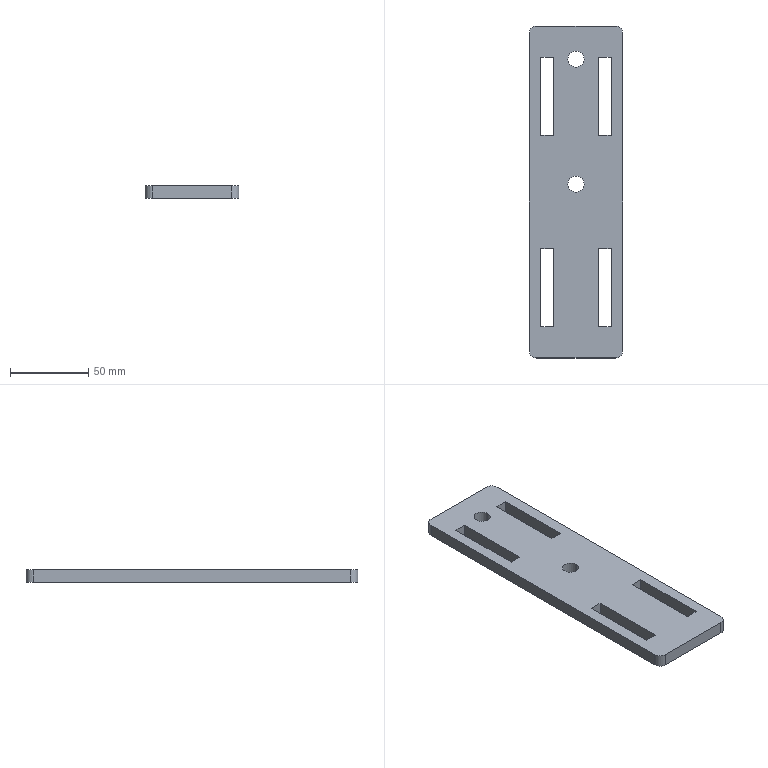Part | SolidWorks | features FlatPattern 1, SMBaseFlange 1, SheetMetal 1 | 1 solid | 30 faces | box 60 x 212.5 x 8 mm | volume 87695 mm3 | plane 22 | cylinder 8 | commonest cylinder face diameters 10 x4 10.3 x4
STEP:
#1=CARTESIAN_POINT('',(326.222,40.247,-8.));
#2=VERTEX_POINT('',#1);
#3=CARTESIAN_POINT('',(336.522,40.247,-8.));
#4=VERTEX_POINT('',#3);
#5=CARTESIAN_POINT('',(331.372,40.247,-8.));
#6=DIRECTION('',(0.,0.,1.));
#7=DIRECTION('',(1.,0.,0.));
#8=AXIS2_PLACEMENT_3D('',#5,#6,#7);
#9=CIRCLE('',#8,5.15);
#10=EDGE_CURVE('',#2,#4,#9,.T.);
#11=ORIENTED_EDGE('',*,*,#10,.F.);
#12=CARTESIAN_POINT('',(326.222,40.247,0.));
#13=VERTEX_POINT('',#12);
#14=CARTESIAN_POINT('',(326.222,40.247,-8.));
#15=DIRECTION('',(0.,0.,1.));
#16=VECTOR('',#15,1000.);
#17=LINE('',#14,#16);
#18=EDGE_CURVE('',#2,#13,#17,.T.);
#19=ORIENTED_EDGE('',*,*,#18,.T.);
#20=CARTESIAN_POINT('',(336.522,40.247,0.));
#21=VERTEX_POINT('',#20);
#22=CARTESIAN_POINT('',(331.372,40.247,0.));
#23=DIRECTION('',(0.,0.,1.));
#24=DIRECTION('',(1.,0.,0.));
#25=AXIS2_PLACEMENT_3D('',#22,#23,#24);
#26=CIRCLE('',#25,5.15);
#27=EDGE_CURVE('',#13,#21,#26,.T.);
#28=ORIENTED_EDGE('',*,*,#27,.T.);
#29=CARTESIAN_POINT('',(336.522,40.247,-8.));
#30=DIRECTION('',(0.,0.,1.));
#31=VECTOR('',#30,1000.);
#32=LINE('',#29,#31);
#33=EDGE_CURVE('',#4,#21,#32,.T.);
#34=ORIENTED_EDGE('',*,*,#33,.F.);
#35=EDGE_LOOP('',(#11,#19,#28,#34));
#36=FACE_OUTER_BOUND('',#35,.T.);
#37=CARTESIAN_POINT('',(331.372,40.247,-8.));
#38=DIRECTION('',(0.,0.,1.));
#39=DIRECTION('',(1.,0.,0.));
#40=AXIS2_PLACEMENT_3D('',#37,#38,#39);
#41=CYLINDRICAL_SURFACE('',#40,5.15);
#42=ADVANCED_FACE('',(#36),#41,.F.);
#43=CARTESIAN_POINT('',(326.222,-39.753,-8.));
#44=VERTEX_POINT('',#43);
#45=CARTESIAN_POINT('',(336.522,-39.753,-8.));
#46=VERTEX_POINT('',#45);
#47=CARTESIAN_POINT('',(331.372,-39.753,-8.));
#48=DIRECTION('',(0.,0.,1.));
#49=DIRECTION('',(1.,0.,0.));
#50=AXIS2_PLACEMENT_3D('',#47,#48,#49);
#51=CIRCLE('',#50,5.15);
#52=EDGE_CURVE('',#44,#46,#51,.T.);
#53=ORIENTED_EDGE('',*,*,#52,.F.);
#54=CARTESIAN_POINT('',(326.222,-39.753,0.));
#55=VERTEX_POINT('',#54);
#56=CARTESIAN_POINT('',(326.222,-39.753,-8.));
#57=DIRECTION('',(0.,0.,1.));
#58=VECTOR('',#57,1000.);
#59=LINE('',#56,#58);
#60=EDGE_CURVE('',#44,#55,#59,.T.);
#61=ORIENTED_EDGE('',*,*,#60,.T.);
#62=CARTESIAN_POINT('',(336.522,-39.753,0.));
#63=VERTEX_POINT('',#62);
#64=CARTESIAN_POINT('',(331.372,-39.753,0.));
#65=DIRECTION('',(0.,0.,1.));
#66=DIRECTION('',(1.,0.,0.));
#67=AXIS2_PLACEMENT_3D('',#64,#65,#66);
#68=CIRCLE('',#67,5.15);
#69=EDGE_CURVE('',#55,#63,#68,.T.);
#70=ORIENTED_EDGE('',*,*,#69,.T.);
#71=CARTESIAN_POINT('',(336.522,-39.753,-8.));
#72=DIRECTION('',(0.,0.,1.));
#73=VECTOR('',#72,1000.);
#74=LINE('',#71,#73);
#75=EDGE_CURVE('',#46,#63,#74,.T.);
#76=ORIENTED_EDGE('',*,*,#75,.F.);
#77=EDGE_LOOP('',(#53,#61,#70,#76));
#78=FACE_OUTER_BOUND('',#77,.T.);
#79=CARTESIAN_POINT('',(331.372,-39.753,-8.));
#80=DIRECTION('',(0.,0.,1.));
#81=DIRECTION('',(1.,0.,0.));
#82=AXIS2_PLACEMENT_3D('',#79,#80,#81);
#83=CYLINDRICAL_SURFACE('',#82,5.15);
#84=ADVANCED_FACE('',(#78),#83,.F.);
#85=CARTESIAN_POINT('',(356.372,-151.003,0.));
#86=VERTEX_POINT('',#85);
#87=CARTESIAN_POINT('',(361.372,-146.003,0.));
#88=VERTEX_POINT('',#87);
#89=CARTESIAN_POINT('',(356.372,-146.003,0.));
#90=DIRECTION('',(0.,0.,1.));
#91=DIRECTION('',(1.,0.,0.));
#92=AXIS2_PLACEMENT_3D('',#89,#90,#91);
#93=CIRCLE('',#92,5.);
#94=EDGE_CURVE('',#86,#88,#93,.T.);
#95=ORIENTED_EDGE('',*,*,#94,.F.);
#96=CARTESIAN_POINT('',(356.372,-151.003,-8.));
#97=VERTEX_POINT('',#96);
#98=CARTESIAN_POINT('',(356.372,-151.003,-8.));
#99=DIRECTION('',(0.,0.,1.));
#100=VECTOR('',#99,1000.);
#101=LINE('',#98,#100);
#102=EDGE_CURVE('',#97,#86,#101,.T.);
#103=ORIENTED_EDGE('',*,*,#102,.F.);
#104=CARTESIAN_POINT('',(361.372,-146.003,-8.));
#105=VERTEX_POINT('',#104);
#106=CARTESIAN_POINT('',(356.372,-146.003,-8.));
#107=DIRECTION('',(0.,0.,1.));
#108=DIRECTION('',(1.,0.,0.));
#109=AXIS2_PLACEMENT_3D('',#106,#107,#108);
#110=CIRCLE('',#109,5.);
#111=EDGE_CURVE('',#97,#105,#110,.T.);
#112=ORIENTED_EDGE('',*,*,#111,.T.);
#113=CARTESIAN_POINT('',(361.372,-146.003,-8.));
#114=DIRECTION('',(0.,0.,1.));
#115=VECTOR('',#114,1000.);
#116=LINE('',#113,#115);
#117=EDGE_CURVE('',#105,#88,#116,.T.);
#118=ORIENTED_EDGE('',*,*,#117,.T.);
#119=EDGE_LOOP('',(#95,#103,#112,#118));
#120=FACE_OUTER_BOUND('',#119,.T.);
#121=CARTESIAN_POINT('',(356.372,-146.003,-8.));
#122=DIRECTION('',(0.,0.,1.));
#123=DIRECTION('',(1.,0.,0.));
#124=AXIS2_PLACEMENT_3D('',#121,#122,#123);
#125=CYLINDRICAL_SURFACE('',#124,5.);
#126=ADVANCED_FACE('',(#120),#125,.T.);
#127=CARTESIAN_POINT('',(306.372,-151.003,0.));
#128=VERTEX_POINT('',#127);
#129=CARTESIAN_POINT('',(306.372,-151.003,0.));
#130=DIRECTION('',(1.,0.,0.));
#131=VECTOR('',#130,1000.);
#132=LINE('',#129,#131);
#133=EDGE_CURVE('',#128,#86,#132,.T.);
#134=ORIENTED_EDGE('',*,*,#133,.F.);
#135=CARTESIAN_POINT('',(306.372,-151.003,-8.));
#136=VERTEX_POINT('',#135);
#137=CARTESIAN_POINT('',(306.372,-151.003,-8.));
#138=DIRECTION('',(0.,0.,1.));
#139=VECTOR('',#138,1000.);
#140=LINE('',#137,#139);
#141=EDGE_CURVE('',#136,#128,#140,.T.);
#142=ORIENTED_EDGE('',*,*,#141,.F.);
#143=CARTESIAN_POINT('',(306.372,-151.003,-8.));
#144=DIRECTION('',(1.,0.,0.));
#145=VECTOR('',#144,1000.);
#146=LINE('',#143,#145);
#147=EDGE_CURVE('',#136,#97,#146,.T.);
#148=ORIENTED_EDGE('',*,*,#147,.T.);
#149=ORIENTED_EDGE('',*,*,#102,.T.);
#150=EDGE_LOOP('',(#134,#142,#148,#149));
#151=FACE_OUTER_BOUND('',#150,.T.);
#152=CARTESIAN_POINT('',(306.372,-151.003,-8.));
#153=DIRECTION('',(0.,-1.,0.));
#154=DIRECTION('',(1.,0.,0.));
#155=AXIS2_PLACEMENT_3D('',#152,#153,#154);
#156=PLANE('',#155);
#157=ADVANCED_FACE('',(#151),#156,.T.);
#158=CARTESIAN_POINT('',(301.372,-146.003,0.));
#159=VERTEX_POINT('',#158);
#160=CARTESIAN_POINT('',(306.372,-146.003,0.));
#161=DIRECTION('',(0.,0.,1.));
#162=DIRECTION('',(-1.,0.,0.));
#163=AXIS2_PLACEMENT_3D('',#160,#161,#162);
#164=CIRCLE('',#163,5.);
#165=EDGE_CURVE('',#159,#128,#164,.T.);
#166=ORIENTED_EDGE('',*,*,#165,.F.);
#167=CARTESIAN_POINT('',(301.372,-146.003,-8.));
#168=VERTEX_POINT('',#167);
#169=CARTESIAN_POINT('',(301.372,-146.003,-8.));
#170=DIRECTION('',(0.,0.,1.));
#171=VECTOR('',#170,1000.);
#172=LINE('',#169,#171);
#173=EDGE_CURVE('',#168,#159,#172,.T.);
#174=ORIENTED_EDGE('',*,*,#173,.F.);
#175=CARTESIAN_POINT('',(306.372,-146.003,-8.));
#176=DIRECTION('',(0.,0.,1.));
#177=DIRECTION('',(-1.,0.,0.));
#178=AXIS2_PLACEMENT_3D('',#175,#176,#177);
#179=CIRCLE('',#178,5.);
#180=EDGE_CURVE('',#168,#136,#179,.T.);
#181=ORIENTED_EDGE('',*,*,#180,.T.);
#182=ORIENTED_EDGE('',*,*,#141,.T.);
#183=EDGE_LOOP('',(#166,#174,#181,#182));
#184=FACE_OUTER_BOUND('',#183,.T.);
#185=CARTESIAN_POINT('',(306.372,-146.003,-8.));
#186=DIRECTION('',(0.,0.,1.));
#187=DIRECTION('',(1.,0.,0.));
#188=AXIS2_PLACEMENT_3D('',#185,#186,#187);
#189=CYLINDRICAL_SURFACE('',#188,5.);
#190=ADVANCED_FACE('',(#184),#189,.T.);
#191=CARTESIAN_POINT('',(301.372,56.497,0.));
#192=VERTEX_POINT('',#191);
#193=CARTESIAN_POINT('',(301.372,-146.003,0.));
#194=DIRECTION('',(0.,-1.,0.));
#195=VECTOR('',#194,1000.);
#196=LINE('',#193,#195);
#197=EDGE_CURVE('',#192,#159,#196,.T.);
#198=ORIENTED_EDGE('',*,*,#197,.F.);
#199=CARTESIAN_POINT('',(301.372,56.497,-8.));
#200=VERTEX_POINT('',#199);
#201=CARTESIAN_POINT('',(301.372,56.497,-8.));
#202=DIRECTION('',(0.,0.,1.));
#203=VECTOR('',#202,1000.);
#204=LINE('',#201,#203);
#205=EDGE_CURVE('',#200,#192,#204,.T.);
#206=ORIENTED_EDGE('',*,*,#205,.F.);
#207=CARTESIAN_POINT('',(301.372,-146.003,-8.));
#208=DIRECTION('',(0.,-1.,0.));
#209=VECTOR('',#208,1000.);
#210=LINE('',#207,#209);
#211=EDGE_CURVE('',#200,#168,#210,.T.);
#212=ORIENTED_EDGE('',*,*,#211,.T.);
#213=ORIENTED_EDGE('',*,*,#173,.T.);
#214=EDGE_LOOP('',(#198,#206,#212,#213));
#215=FACE_OUTER_BOUND('',#214,.T.);
#216=CARTESIAN_POINT('',(301.372,-146.003,-8.));
#217=DIRECTION('',(-1.,0.,0.));
#218=DIRECTION('',(0.,0.,1.));
#219=AXIS2_PLACEMENT_3D('',#216,#217,#218);
#220=PLANE('',#219);
#221=ADVANCED_FACE('',(#215),#220,.T.);
#222=CARTESIAN_POINT('',(306.372,61.497,0.));
#223=VERTEX_POINT('',#222);
#224=CARTESIAN_POINT('',(306.372,56.497,0.));
#225=DIRECTION('',(0.,0.,1.));
#226=DIRECTION('',(-1.,0.,0.));
#227=AXIS2_PLACEMENT_3D('',#224,#225,#226);
#228=CIRCLE('',#227,5.);
#229=EDGE_CURVE('',#223,#192,#228,.T.);
#230=ORIENTED_EDGE('',*,*,#229,.F.);
#231=CARTESIAN_POINT('',(306.372,61.497,-8.));
#232=VERTEX_POINT('',#231);
#233=CARTESIAN_POINT('',(306.372,61.497,-8.));
#234=DIRECTION('',(0.,0.,1.));
#235=VECTOR('',#234,1000.);
#236=LINE('',#233,#235);
#237=EDGE_CURVE('',#232,#223,#236,.T.);
#238=ORIENTED_EDGE('',*,*,#237,.F.);
#239=CARTESIAN_POINT('',(306.372,56.497,-8.));
#240=DIRECTION('',(0.,0.,1.));
#241=DIRECTION('',(-1.,0.,0.));
#242=AXIS2_PLACEMENT_3D('',#239,#240,#241);
#243=CIRCLE('',#242,5.);
#244=EDGE_CURVE('',#232,#200,#243,.T.);
#245=ORIENTED_EDGE('',*,*,#244,.T.);
#246=ORIENTED_EDGE('',*,*,#205,.T.);
#247=EDGE_LOOP('',(#230,#238,#245,#246));
#248=FACE_OUTER_BOUND('',#247,.T.);
#249=CARTESIAN_POINT('',(306.372,56.497,-8.));
#250=DIRECTION('',(0.,0.,1.));
#251=DIRECTION('',(1.,0.,0.));
#252=AXIS2_PLACEMENT_3D('',#249,#250,#251);
#253=CYLINDRICAL_SURFACE('',#252,5.);
#254=ADVANCED_FACE('',(#248),#253,.T.);
#255=CARTESIAN_POINT('',(356.372,61.497,0.));
#256=VERTEX_POINT('',#255);
#257=CARTESIAN_POINT('',(306.372,61.497,0.));
#258=DIRECTION('',(-1.,0.,0.));
#259=VECTOR('',#258,1000.);
#260=LINE('',#257,#259);
#261=EDGE_CURVE('',#256,#223,#260,.T.);
#262=ORIENTED_EDGE('',*,*,#261,.F.);
#263=CARTESIAN_POINT('',(356.372,61.497,-8.));
#264=VERTEX_POINT('',#263);
#265=CARTESIAN_POINT('',(356.372,61.497,-8.));
#266=DIRECTION('',(0.,0.,1.));
#267=VECTOR('',#266,1000.);
#268=LINE('',#265,#267);
#269=EDGE_CURVE('',#264,#256,#268,.T.);
#270=ORIENTED_EDGE('',*,*,#269,.F.);
#271=CARTESIAN_POINT('',(306.372,61.497,-8.));
#272=DIRECTION('',(-1.,0.,0.));
#273=VECTOR('',#272,1000.);
#274=LINE('',#271,#273);
#275=EDGE_CURVE('',#264,#232,#274,.T.);
#276=ORIENTED_EDGE('',*,*,#275,.T.);
#277=ORIENTED_EDGE('',*,*,#237,.T.);
#278=EDGE_LOOP('',(#262,#270,#276,#277));
#279=FACE_OUTER_BOUND('',#278,.T.);
#280=CARTESIAN_POINT('',(306.372,61.497,-8.));
#281=DIRECTION('',(0.,1.,0.));
#282=DIRECTION('',(0.,0.,1.));
#283=AXIS2_PLACEMENT_3D('',#280,#281,#282);
#284=PLANE('',#283);
#285=ADVANCED_FACE('',(#279),#284,.T.);
#286=CARTESIAN_POINT('',(361.372,56.497,0.));
#287=VERTEX_POINT('',#286);
#288=CARTESIAN_POINT('',(356.372,56.497,0.));
#289=DIRECTION('',(0.,0.,1.));
#290=DIRECTION('',(-1.,0.,0.));
#291=AXIS2_PLACEMENT_3D('',#288,#289,#290);
#292=CIRCLE('',#291,5.);
#293=EDGE_CURVE('',#287,#256,#292,.T.);
#294=ORIENTED_EDGE('',*,*,#293,.F.);
#295=CARTESIAN_POINT('',(361.372,56.497,-8.));
#296=VERTEX_POINT('',#295);
#297=CARTESIAN_POINT('',(361.372,56.497,-8.));
#298=DIRECTION('',(0.,0.,1.));
#299=VECTOR('',#298,1000.);
#300=LINE('',#297,#299);
#301=EDGE_CURVE('',#296,#287,#300,.T.);
#302=ORIENTED_EDGE('',*,*,#301,.F.);
#303=CARTESIAN_POINT('',(356.372,56.497,-8.));
#304=DIRECTION('',(0.,0.,1.));
#305=DIRECTION('',(-1.,0.,0.));
#306=AXIS2_PLACEMENT_3D('',#303,#304,#305);
#307=CIRCLE('',#306,5.);
#308=EDGE_CURVE('',#296,#264,#307,.T.);
#309=ORIENTED_EDGE('',*,*,#308,.T.);
#310=ORIENTED_EDGE('',*,*,#269,.T.);
#311=EDGE_LOOP('',(#294,#302,#309,#310));
#312=FACE_OUTER_BOUND('',#311,.T.);
#313=CARTESIAN_POINT('',(356.372,56.497,-8.));
#314=DIRECTION('',(0.,0.,1.));
#315=DIRECTION('',(1.,0.,0.));
#316=AXIS2_PLACEMENT_3D('',#313,#314,#315);
#317=CYLINDRICAL_SURFACE('',#316,5.);
#318=ADVANCED_FACE('',(#312),#317,.T.);
#319=CARTESIAN_POINT('',(361.372,-146.003,0.));
#320=DIRECTION('',(0.,1.,0.));
#321=VECTOR('',#320,1000.);
#322=LINE('',#319,#321);
#323=EDGE_CURVE('',#88,#287,#322,.T.);
#324=ORIENTED_EDGE('',*,*,#323,.F.);
#325=ORIENTED_EDGE('',*,*,#117,.F.);
#326=CARTESIAN_POINT('',(361.372,-146.003,-8.));
#327=DIRECTION('',(0.,1.,0.));
#328=VECTOR('',#327,1000.);
#329=LINE('',#326,#328);
#330=EDGE_CURVE('',#105,#296,#329,.T.);
#331=ORIENTED_EDGE('',*,*,#330,.T.);
#332=ORIENTED_EDGE('',*,*,#301,.T.);
#333=EDGE_LOOP('',(#324,#325,#331,#332));
#334=FACE_OUTER_BOUND('',#333,.T.);
#335=CARTESIAN_POINT('',(361.372,-146.003,-8.));
#336=DIRECTION('',(1.,0.,0.));
#337=DIRECTION('',(0.,0.,-1.));
#338=AXIS2_PLACEMENT_3D('',#335,#336,#337);
#339=PLANE('',#338);
#340=ADVANCED_FACE('',(#334),#339,.T.);
#341=CARTESIAN_POINT('',(345.872,-131.003,-8.));
#342=VERTEX_POINT('',#341);
#343=CARTESIAN_POINT('',(353.872,-131.003,-8.));
#344=VERTEX_POINT('',#343);
#345=CARTESIAN_POINT('',(353.872,-131.003,-8.));
#346=DIRECTION('',(1.,0.,0.));
#347=VECTOR('',#346,1000.);
#348=LINE('',#345,#347);
#349=EDGE_CURVE('',#342,#344,#348,.T.);
#350=ORIENTED_EDGE('',*,*,#349,.T.);
#351=CARTESIAN_POINT('',(353.872,-81.003,-8.));
#352=VERTEX_POINT('',#351);
#353=CARTESIAN_POINT('',(353.872,-81.003,-8.));
#354=DIRECTION('',(0.,1.,0.));
#355=VECTOR('',#354,1000.);
#356=LINE('',#353,#355);
#357=EDGE_CURVE('',#344,#352,#356,.T.);
#358=ORIENTED_EDGE('',*,*,#357,.T.);
#359=CARTESIAN_POINT('',(345.872,-81.003,-8.));
#360=VERTEX_POINT('',#359);
#361=CARTESIAN_POINT('',(353.872,-81.003,-8.));
#362=DIRECTION('',(-1.,0.,0.));
#363=VECTOR('',#362,1000.);
#364=LINE('',#361,#363);
#365=EDGE_CURVE('',#352,#360,#364,.T.);
#366=ORIENTED_EDGE('',*,*,#365,.T.);
#367=CARTESIAN_POINT('',(345.872,-81.003,-8.));
#368=DIRECTION('',(0.,-1.,0.));
#369=VECTOR('',#368,1000.);
#370=LINE('',#367,#369);
#371=EDGE_CURVE('',#360,#342,#370,.T.);
#372=ORIENTED_EDGE('',*,*,#371,.T.);
#373=EDGE_LOOP('',(#350,#358,#366,#372));
#374=FACE_BOUND('',#373,.T.);
#375=CARTESIAN_POINT('',(353.872,41.497,-8.));
#376=VERTEX_POINT('',#375);
#377=CARTESIAN_POINT('',(345.872,41.497,-8.));
#378=VERTEX_POINT('',#377);
#379=CARTESIAN_POINT('',(345.872,41.497,-8.));
#380=DIRECTION('',(-1.,0.,0.));
#381=VECTOR('',#380,1000.);
#382=LINE('',#379,#381);
#383=EDGE_CURVE('',#376,#378,#382,.T.);
#384=ORIENTED_EDGE('',*,*,#383,.T.);
#385=CARTESIAN_POINT('',(345.872,-8.503,-8.));
#386=VERTEX_POINT('',#385);
#387=CARTESIAN_POINT('',(345.872,41.497,-8.));
#388=DIRECTION('',(0.,-1.,0.));
#389=VECTOR('',#388,1000.);
#390=LINE('',#387,#389);
#391=EDGE_CURVE('',#378,#386,#390,.T.);
#392=ORIENTED_EDGE('',*,*,#391,.T.);
#393=CARTESIAN_POINT('',(353.872,-8.503,-8.));
#394=VERTEX_POINT('',#393);
#395=CARTESIAN_POINT('',(345.872,-8.503,-8.));
#396=DIRECTION('',(1.,0.,0.));
#397=VECTOR('',#396,1000.);
#398=LINE('',#395,#397);
#399=EDGE_CURVE('',#386,#394,#398,.T.);
#400=ORIENTED_EDGE('',*,*,#399,.T.);
#401=CARTESIAN_POINT('',(353.872,41.497,-8.));
#402=DIRECTION('',(0.,1.,0.));
#403=VECTOR('',#402,1000.);
#404=LINE('',#401,#403);
#405=EDGE_CURVE('',#394,#376,#404,.T.);
#406=ORIENTED_EDGE('',*,*,#405,.T.);
#407=EDGE_LOOP('',(#384,#392,#400,#406));
#408=FACE_BOUND('',#407,.T.);
#409=CARTESIAN_POINT('',(308.872,-8.503,-8.));
#410=VERTEX_POINT('',#409);
#411=CARTESIAN_POINT('',(316.872,-8.503,-8.));
#412=VERTEX_POINT('',#411);
#413=CARTESIAN_POINT('',(316.872,-8.503,-8.));
#414=DIRECTION('',(1.,0.,0.));
#415=VECTOR('',#414,1000.);
#416=LINE('',#413,#415);
#417=EDGE_CURVE('',#410,#412,#416,.T.);
#418=ORIENTED_EDGE('',*,*,#417,.T.);
#419=CARTESIAN_POINT('',(316.872,41.497,-8.));
#420=VERTEX_POINT('',#419);
#421=CARTESIAN_POINT('',(316.872,-8.503,-8.));
#422=DIRECTION('',(0.,1.,0.));
#423=VECTOR('',#422,1000.);
#424=LINE('',#421,#423);
#425=EDGE_CURVE('',#412,#420,#424,.T.);
#426=ORIENTED_EDGE('',*,*,#425,.T.);
#427=CARTESIAN_POINT('',(308.872,41.497,-8.));
#428=VERTEX_POINT('',#427);
#429=CARTESIAN_POINT('',(316.872,41.497,-8.));
#430=DIRECTION('',(-1.,0.,0.));
#431=VECTOR('',#430,1000.);
#432=LINE('',#429,#431);
#433=EDGE_CURVE('',#420,#428,#432,.T.);
#434=ORIENTED_EDGE('',*,*,#433,.T.);
#435=CARTESIAN_POINT('',(308.872,-8.503,-8.));
#436=DIRECTION('',(0.,-1.,0.));
#437=VECTOR('',#436,1000.);
#438=LINE('',#435,#437);
#439=EDGE_CURVE('',#428,#410,#438,.T.);
#440=ORIENTED_EDGE('',*,*,#439,.T.);
#441=EDGE_LOOP('',(#418,#426,#434,#440));
#442=FACE_BOUND('',#441,.T.);
#443=CARTESIAN_POINT('',(308.872,-131.003,-8.));
#444=VERTEX_POINT('',#443);
#445=CARTESIAN_POINT('',(316.872,-131.003,-8.));
#446=VERTEX_POINT('',#445);
#447=CARTESIAN_POINT('',(316.872,-131.003,-8.));
#448=DIRECTION('',(1.,0.,0.));
#449=VECTOR('',#448,1000.);
#450=LINE('',#447,#449);
#451=EDGE_CURVE('',#444,#446,#450,.T.);
#452=ORIENTED_EDGE('',*,*,#451,.T.);
#453=CARTESIAN_POINT('',(316.872,-81.003,-8.));
#454=VERTEX_POINT('',#453);
#455=CARTESIAN_POINT('',(316.872,-131.003,-8.));
#456=DIRECTION('',(0.,1.,0.));
#457=VECTOR('',#456,1000.);
#458=LINE('',#455,#457);
#459=EDGE_CURVE('',#446,#454,#458,.T.);
#460=ORIENTED_EDGE('',*,*,#459,.T.);
#461=CARTESIAN_POINT('',(308.872,-81.003,-8.));
#462=VERTEX_POINT('',#461);
#463=CARTESIAN_POINT('',(316.872,-81.003,-8.));
#464=DIRECTION('',(-1.,0.,0.));
#465=VECTOR('',#464,1000.);
#466=LINE('',#463,#465);
#467=EDGE_CURVE('',#454,#462,#466,.T.);
#468=ORIENTED_EDGE('',*,*,#467,.T.);
#469=CARTESIAN_POINT('',(308.872,-131.003,-8.));
#470=DIRECTION('',(0.,-1.,0.));
#471=VECTOR('',#470,1000.);
#472=LINE('',#469,#471);
#473=EDGE_CURVE('',#462,#444,#472,.T.);
#474=ORIENTED_EDGE('',*,*,#473,.T.);
#475=EDGE_LOOP('',(#452,#460,#468,#474));
#476=FACE_BOUND('',#475,.T.);
#477=CARTESIAN_POINT('',(331.372,40.247,-8.));
#478=DIRECTION('',(0.,0.,1.));
#479=DIRECTION('',(1.,0.,0.));
#480=AXIS2_PLACEMENT_3D('',#477,#478,#479);
#481=CIRCLE('',#480,5.15);
#482=EDGE_CURVE('',#4,#2,#481,.T.);
#483=ORIENTED_EDGE('',*,*,#482,.T.);
#484=ORIENTED_EDGE('',*,*,#10,.T.);
#485=EDGE_LOOP('',(#483,#484));
#486=FACE_BOUND('',#485,.T.);
#487=CARTESIAN_POINT('',(331.372,-39.753,-8.));
#488=DIRECTION('',(0.,0.,1.));
#489=DIRECTION('',(1.,0.,0.));
#490=AXIS2_PLACEMENT_3D('',#487,#488,#489);
#491=CIRCLE('',#490,5.15);
#492=EDGE_CURVE('',#46,#44,#491,.T.);
#493=ORIENTED_EDGE('',*,*,#492,.T.);
#494=ORIENTED_EDGE('',*,*,#52,.T.);
#495=EDGE_LOOP('',(#493,#494));
#496=FACE_BOUND('',#495,.T.);
#497=ORIENTED_EDGE('',*,*,#111,.F.);
#498=ORIENTED_EDGE('',*,*,#147,.F.);
#499=ORIENTED_EDGE('',*,*,#180,.F.);
#500=ORIENTED_EDGE('',*,*,#211,.F.);
#501=ORIENTED_EDGE('',*,*,#244,.F.);
#502=ORIENTED_EDGE('',*,*,#275,.F.);
#503=ORIENTED_EDGE('',*,*,#308,.F.);
#504=ORIENTED_EDGE('',*,*,#330,.F.);
#505=EDGE_LOOP('',(#497,#498,#499,#500,#501,#502,#503,#504));
#506=FACE_OUTER_BOUND('',#505,.T.);
#507=CARTESIAN_POINT('',(356.372,-146.003,-8.));
#508=DIRECTION('',(0.,0.,1.));
#509=DIRECTION('',(1.,0.,0.));
#510=AXIS2_PLACEMENT_3D('',#507,#508,#509);
#511=PLANE('',#510);
#512=ADVANCED_FACE('',(#374,#408,#442,#476,#486,#496,#506),#511,.F.);
#513=CARTESIAN_POINT('',(353.872,-131.003,0.));
#514=VERTEX_POINT('',#513);
#515=CARTESIAN_POINT('',(353.872,-81.003,0.));
#516=VERTEX_POINT('',#515);
#517=CARTESIAN_POINT('',(353.872,-81.003,0.));
#518=DIRECTION('',(0.,1.,0.));
#519=VECTOR('',#518,1000.);
#520=LINE('',#517,#519);
#521=EDGE_CURVE('',#514,#516,#520,.T.);
#522=ORIENTED_EDGE('',*,*,#521,.F.);
#523=CARTESIAN_POINT('',(345.872,-131.003,0.));
#524=VERTEX_POINT('',#523);
#525=CARTESIAN_POINT('',(353.872,-131.003,0.));
#526=DIRECTION('',(1.,0.,0.));
#527=VECTOR('',#526,1000.);
#528=LINE('',#525,#527);
#529=EDGE_CURVE('',#524,#514,#528,.T.);
#530=ORIENTED_EDGE('',*,*,#529,.F.);
#531=CARTESIAN_POINT('',(345.872,-81.003,0.));
#532=VERTEX_POINT('',#531);
#533=CARTESIAN_POINT('',(345.872,-81.003,0.));
#534=DIRECTION('',(0.,-1.,0.));
#535=VECTOR('',#534,1000.);
#536=LINE('',#533,#535);
#537=EDGE_CURVE('',#532,#524,#536,.T.);
#538=ORIENTED_EDGE('',*,*,#537,.F.);
#539=CARTESIAN_POINT('',(353.872,-81.003,0.));
#540=DIRECTION('',(-1.,0.,0.));
#541=VECTOR('',#540,1000.);
#542=LINE('',#539,#541);
#543=EDGE_CURVE('',#516,#532,#542,.T.);
#544=ORIENTED_EDGE('',*,*,#543,.F.);
#545=EDGE_LOOP('',(#522,#530,#538,#544));
#546=FACE_BOUND('',#545,.T.);
#547=CARTESIAN_POINT('',(345.872,41.497,0.));
#548=VERTEX_POINT('',#547);
#549=CARTESIAN_POINT('',(345.872,-8.503,0.));
#550=VERTEX_POINT('',#549);
#551=CARTESIAN_POINT('',(345.872,41.497,0.));
#552=DIRECTION('',(0.,-1.,0.));
#553=VECTOR('',#552,1000.);
#554=LINE('',#551,#553);
#555=EDGE_CURVE('',#548,#550,#554,.T.);
#556=ORIENTED_EDGE('',*,*,#555,.F.);
#557=CARTESIAN_POINT('',(353.872,41.497,0.));
#558=VERTEX_POINT('',#557);
#559=CARTESIAN_POINT('',(345.872,41.497,0.));
#560=DIRECTION('',(-1.,0.,0.));
#561=VECTOR('',#560,1000.);
#562=LINE('',#559,#561);
#563=EDGE_CURVE('',#558,#548,#562,.T.);
#564=ORIENTED_EDGE('',*,*,#563,.F.);
#565=CARTESIAN_POINT('',(353.872,-8.503,0.));
#566=VERTEX_POINT('',#565);
#567=CARTESIAN_POINT('',(353.872,41.497,0.));
#568=DIRECTION('',(0.,1.,0.));
#569=VECTOR('',#568,1000.);
#570=LINE('',#567,#569);
#571=EDGE_CURVE('',#566,#558,#570,.T.);
#572=ORIENTED_EDGE('',*,*,#571,.F.);
#573=CARTESIAN_POINT('',(345.872,-8.503,0.));
#574=DIRECTION('',(1.,0.,0.));
#575=VECTOR('',#574,1000.);
#576=LINE('',#573,#575);
#577=EDGE_CURVE('',#550,#566,#576,.T.);
#578=ORIENTED_EDGE('',*,*,#577,.F.);
#579=EDGE_LOOP('',(#556,#564,#572,#578));
#580=FACE_BOUND('',#579,.T.);
#581=CARTESIAN_POINT('',(316.872,-8.503,0.));
#582=VERTEX_POINT('',#581);
#583=CARTESIAN_POINT('',(316.872,41.497,0.));
#584=VERTEX_POINT('',#583);
#585=CARTESIAN_POINT('',(316.872,-8.503,0.));
#586=DIRECTION('',(0.,1.,0.));
#587=VECTOR('',#586,1000.);
#588=LINE('',#585,#587);
#589=EDGE_CURVE('',#582,#584,#588,.T.);
#590=ORIENTED_EDGE('',*,*,#589,.F.);
#591=CARTESIAN_POINT('',(308.872,-8.503,0.));
#592=VERTEX_POINT('',#591);
#593=CARTESIAN_POINT('',(316.872,-8.503,0.));
#594=DIRECTION('',(1.,0.,0.));
#595=VECTOR('',#594,1000.);
#596=LINE('',#593,#595);
#597=EDGE_CURVE('',#592,#582,#596,.T.);
#598=ORIENTED_EDGE('',*,*,#597,.F.);
#599=CARTESIAN_POINT('',(308.872,41.497,0.));
#600=VERTEX_POINT('',#599);
#601=CARTESIAN_POINT('',(308.872,-8.503,0.));
#602=DIRECTION('',(0.,-1.,0.));
#603=VECTOR('',#602,1000.);
#604=LINE('',#601,#603);
#605=EDGE_CURVE('',#600,#592,#604,.T.);
#606=ORIENTED_EDGE('',*,*,#605,.F.);
#607=CARTESIAN_POINT('',(316.872,41.497,0.));
#608=DIRECTION('',(-1.,0.,0.));
#609=VECTOR('',#608,1000.);
#610=LINE('',#607,#609);
#611=EDGE_CURVE('',#584,#600,#610,.T.);
#612=ORIENTED_EDGE('',*,*,#611,.F.);
#613=EDGE_LOOP('',(#590,#598,#606,#612));
#614=FACE_BOUND('',#613,.T.);
#615=CARTESIAN_POINT('',(316.872,-131.003,0.));
#616=VERTEX_POINT('',#615);
#617=CARTESIAN_POINT('',(316.872,-81.003,0.));
#618=VERTEX_POINT('',#617);
#619=CARTESIAN_POINT('',(316.872,-131.003,0.));
#620=DIRECTION('',(0.,1.,0.));
#621=VECTOR('',#620,1000.);
#622=LINE('',#619,#621);
#623=EDGE_CURVE('',#616,#618,#622,.T.);
#624=ORIENTED_EDGE('',*,*,#623,.F.);
#625=CARTESIAN_POINT('',(308.872,-131.003,0.));
#626=VERTEX_POINT('',#625);
#627=CARTESIAN_POINT('',(316.872,-131.003,0.));
#628=DIRECTION('',(1.,0.,0.));
#629=VECTOR('',#628,1000.);
#630=LINE('',#627,#629);
#631=EDGE_CURVE('',#626,#616,#630,.T.);
#632=ORIENTED_EDGE('',*,*,#631,.F.);
#633=CARTESIAN_POINT('',(308.872,-81.003,0.));
#634=VERTEX_POINT('',#633);
#635=CARTESIAN_POINT('',(308.872,-131.003,0.));
#636=DIRECTION('',(0.,-1.,0.));
#637=VECTOR('',#636,1000.);
#638=LINE('',#635,#637);
#639=EDGE_CURVE('',#634,#626,#638,.T.);
#640=ORIENTED_EDGE('',*,*,#639,.F.);
#641=CARTESIAN_POINT('',(316.872,-81.003,0.));
#642=DIRECTION('',(-1.,0.,0.));
#643=VECTOR('',#642,1000.);
#644=LINE('',#641,#643);
#645=EDGE_CURVE('',#618,#634,#644,.T.);
#646=ORIENTED_EDGE('',*,*,#645,.F.);
#647=EDGE_LOOP('',(#624,#632,#640,#646));
#648=FACE_BOUND('',#647,.T.);
#649=CARTESIAN_POINT('',(331.372,40.247,0.));
#650=DIRECTION('',(0.,0.,1.));
#651=DIRECTION('',(1.,0.,0.));
#652=AXIS2_PLACEMENT_3D('',#649,#650,#651);
#653=CIRCLE('',#652,5.15);
#654=EDGE_CURVE('',#21,#13,#653,.T.);
#655=ORIENTED_EDGE('',*,*,#654,.F.);
#656=ORIENTED_EDGE('',*,*,#27,.F.);
#657=EDGE_LOOP('',(#655,#656));
#658=FACE_BOUND('',#657,.T.);
#659=CARTESIAN_POINT('',(331.372,-39.753,0.));
#660=DIRECTION('',(0.,0.,1.));
#661=DIRECTION('',(1.,0.,0.));
#662=AXIS2_PLACEMENT_3D('',#659,#660,#661);
#663=CIRCLE('',#662,5.15);
#664=EDGE_CURVE('',#63,#55,#663,.T.);
#665=ORIENTED_EDGE('',*,*,#664,.F.);
#666=ORIENTED_EDGE('',*,*,#69,.F.);
#667=EDGE_LOOP('',(#665,#666));
#668=FACE_BOUND('',#667,.T.);
#669=ORIENTED_EDGE('',*,*,#94,.T.);
#670=ORIENTED_EDGE('',*,*,#323,.T.);
#671=ORIENTED_EDGE('',*,*,#293,.T.);
#672=ORIENTED_EDGE('',*,*,#261,.T.);
#673=ORIENTED_EDGE('',*,*,#229,.T.);
#674=ORIENTED_EDGE('',*,*,#197,.T.);
#675=ORIENTED_EDGE('',*,*,#165,.T.);
#676=ORIENTED_EDGE('',*,*,#133,.T.);
#677=EDGE_LOOP('',(#669,#670,#671,#672,#673,#674,#675,#676));
#678=FACE_OUTER_BOUND('',#677,.T.);
#679=CARTESIAN_POINT('',(356.372,-146.003,0.));
#680=DIRECTION('',(0.,0.,1.));
#681=DIRECTION('',(1.,0.,0.));
#682=AXIS2_PLACEMENT_3D('',#679,#680,#681);
#683=PLANE('',#682);
#684=ADVANCED_FACE('',(#546,#580,#614,#648,#658,#668,#678),#683,.T.);
#685=ORIENTED_EDGE('',*,*,#60,.F.);
#686=ORIENTED_EDGE('',*,*,#492,.F.);
#687=ORIENTED_EDGE('',*,*,#75,.T.);
#688=ORIENTED_EDGE('',*,*,#664,.T.);
#689=EDGE_LOOP('',(#685,#686,#687,#688));
#690=FACE_OUTER_BOUND('',#689,.T.);
#691=CARTESIAN_POINT('',(331.372,-39.753,-8.));
#692=DIRECTION('',(0.,0.,1.));
#693=DIRECTION('',(1.,0.,0.));
#694=AXIS2_PLACEMENT_3D('',#691,#692,#693);
#695=CYLINDRICAL_SURFACE('',#694,5.15);
#696=ADVANCED_FACE('',(#690),#695,.F.);
#697=ORIENTED_EDGE('',*,*,#18,.F.);
#698=ORIENTED_EDGE('',*,*,#482,.F.);
#699=ORIENTED_EDGE('',*,*,#33,.T.);
#700=ORIENTED_EDGE('',*,*,#654,.T.);
#701=EDGE_LOOP('',(#697,#698,#699,#700));
#702=FACE_OUTER_BOUND('',#701,.T.);
#703=CARTESIAN_POINT('',(331.372,40.247,-8.));
#704=DIRECTION('',(0.,0.,1.));
#705=DIRECTION('',(1.,0.,0.));
#706=AXIS2_PLACEMENT_3D('',#703,#704,#705);
#707=CYLINDRICAL_SURFACE('',#706,5.15);
#708=ADVANCED_FACE('',(#702),#707,.F.);
#709=ORIENTED_EDGE('',*,*,#623,.T.);
#710=CARTESIAN_POINT('',(316.872,-81.003,-8.));
#711=DIRECTION('',(0.,0.,1.));
#712=VECTOR('',#711,1000.);
#713=LINE('',#710,#712);
#714=EDGE_CURVE('',#454,#618,#713,.T.);
#715=ORIENTED_EDGE('',*,*,#714,.F.);
#716=ORIENTED_EDGE('',*,*,#459,.F.);
#717=CARTESIAN_POINT('',(316.872,-131.003,-8.));
#718=DIRECTION('',(0.,0.,1.));
#719=VECTOR('',#718,1000.);
#720=LINE('',#717,#719);
#721=EDGE_CURVE('',#446,#616,#720,.T.);
#722=ORIENTED_EDGE('',*,*,#721,.T.);
#723=EDGE_LOOP('',(#709,#715,#716,#722));
#724=FACE_OUTER_BOUND('',#723,.T.);
#725=CARTESIAN_POINT('',(316.872,-131.003,-8.));
#726=DIRECTION('',(1.,0.,0.));
#727=DIRECTION('',(0.,0.,-1.));
#728=AXIS2_PLACEMENT_3D('',#725,#726,#727);
#729=PLANE('',#728);
#730=ADVANCED_FACE('',(#724),#729,.F.);
#731=ORIENTED_EDGE('',*,*,#631,.T.);
#732=ORIENTED_EDGE('',*,*,#721,.F.);
#733=ORIENTED_EDGE('',*,*,#451,.F.);
#734=CARTESIAN_POINT('',(308.872,-131.003,-8.));
#735=DIRECTION('',(0.,0.,1.));
#736=VECTOR('',#735,1000.);
#737=LINE('',#734,#736);
#738=EDGE_CURVE('',#444,#626,#737,.T.);
#739=ORIENTED_EDGE('',*,*,#738,.T.);
#740=EDGE_LOOP('',(#731,#732,#733,#739));
#741=FACE_OUTER_BOUND('',#740,.T.);
#742=CARTESIAN_POINT('',(316.872,-131.003,-8.));
#743=DIRECTION('',(0.,-1.,0.));
#744=DIRECTION('',(1.,0.,0.));
#745=AXIS2_PLACEMENT_3D('',#742,#743,#744);
#746=PLANE('',#745);
#747=ADVANCED_FACE('',(#741),#746,.F.);
#748=ORIENTED_EDGE('',*,*,#639,.T.);
#749=ORIENTED_EDGE('',*,*,#738,.F.);
#750=ORIENTED_EDGE('',*,*,#473,.F.);
#751=CARTESIAN_POINT('',(308.872,-81.003,-8.));
#752=DIRECTION('',(0.,0.,1.));
#753=VECTOR('',#752,1000.);
#754=LINE('',#751,#753);
#755=EDGE_CURVE('',#462,#634,#754,.T.);
#756=ORIENTED_EDGE('',*,*,#755,.T.);
#757=EDGE_LOOP('',(#748,#749,#750,#756));
#758=FACE_OUTER_BOUND('',#757,.T.);
#759=CARTESIAN_POINT('',(308.872,-131.003,-8.));
#760=DIRECTION('',(-1.,0.,0.));
#761=DIRECTION('',(0.,0.,1.));
#762=AXIS2_PLACEMENT_3D('',#759,#760,#761);
#763=PLANE('',#762);
#764=ADVANCED_FACE('',(#758),#763,.F.);
#765=ORIENTED_EDGE('',*,*,#645,.T.);
#766=ORIENTED_EDGE('',*,*,#755,.F.);
#767=ORIENTED_EDGE('',*,*,#467,.F.);
#768=ORIENTED_EDGE('',*,*,#714,.T.);
#769=EDGE_LOOP('',(#765,#766,#767,#768));
#770=FACE_OUTER_BOUND('',#769,.T.);
#771=CARTESIAN_POINT('',(316.872,-81.003,-8.));
#772=DIRECTION('',(0.,1.,0.));
#773=DIRECTION('',(0.,0.,1.));
#774=AXIS2_PLACEMENT_3D('',#771,#772,#773);
#775=PLANE('',#774);
#776=ADVANCED_FACE('',(#770),#775,.F.);
#777=ORIENTED_EDGE('',*,*,#589,.T.);
#778=CARTESIAN_POINT('',(316.872,41.497,-8.));
#779=DIRECTION('',(0.,0.,1.));
#780=VECTOR('',#779,1000.);
#781=LINE('',#778,#780);
#782=EDGE_CURVE('',#420,#584,#781,.T.);
#783=ORIENTED_EDGE('',*,*,#782,.F.);
#784=ORIENTED_EDGE('',*,*,#425,.F.);
#785=CARTESIAN_POINT('',(316.872,-8.503,-8.));
#786=DIRECTION('',(0.,0.,1.));
#787=VECTOR('',#786,1000.);
#788=LINE('',#785,#787);
#789=EDGE_CURVE('',#412,#582,#788,.T.);
#790=ORIENTED_EDGE('',*,*,#789,.T.);
#791=EDGE_LOOP('',(#777,#783,#784,#790));
#792=FACE_OUTER_BOUND('',#791,.T.);
#793=CARTESIAN_POINT('',(316.872,-8.503,-8.));
#794=DIRECTION('',(1.,0.,0.));
#795=DIRECTION('',(0.,0.,-1.));
#796=AXIS2_PLACEMENT_3D('',#793,#794,#795);
#797=PLANE('',#796);
#798=ADVANCED_FACE('',(#792),#797,.F.);
#799=ORIENTED_EDGE('',*,*,#597,.T.);
#800=ORIENTED_EDGE('',*,*,#789,.F.);
#801=ORIENTED_EDGE('',*,*,#417,.F.);
#802=CARTESIAN_POINT('',(308.872,-8.503,-8.));
#803=DIRECTION('',(0.,0.,1.));
#804=VECTOR('',#803,1000.);
#805=LINE('',#802,#804);
#806=EDGE_CURVE('',#410,#592,#805,.T.);
#807=ORIENTED_EDGE('',*,*,#806,.T.);
#808=EDGE_LOOP('',(#799,#800,#801,#807));
#809=FACE_OUTER_BOUND('',#808,.T.);
#810=CARTESIAN_POINT('',(316.872,-8.503,-8.));
#811=DIRECTION('',(0.,-1.,0.));
#812=DIRECTION('',(1.,0.,0.));
#813=AXIS2_PLACEMENT_3D('',#810,#811,#812);
#814=PLANE('',#813);
#815=ADVANCED_FACE('',(#809),#814,.F.);
#816=ORIENTED_EDGE('',*,*,#605,.T.);
#817=ORIENTED_EDGE('',*,*,#806,.F.);
#818=ORIENTED_EDGE('',*,*,#439,.F.);
#819=CARTESIAN_POINT('',(308.872,41.497,-8.));
#820=DIRECTION('',(0.,0.,1.));
#821=VECTOR('',#820,1000.);
#822=LINE('',#819,#821);
#823=EDGE_CURVE('',#428,#600,#822,.T.);
#824=ORIENTED_EDGE('',*,*,#823,.T.);
#825=EDGE_LOOP('',(#816,#817,#818,#824));
#826=FACE_OUTER_BOUND('',#825,.T.);
#827=CARTESIAN_POINT('',(308.872,-8.503,-8.));
#828=DIRECTION('',(-1.,0.,0.));
#829=DIRECTION('',(0.,0.,1.));
#830=AXIS2_PLACEMENT_3D('',#827,#828,#829);
#831=PLANE('',#830);
#832=ADVANCED_FACE('',(#826),#831,.F.);
#833=ORIENTED_EDGE('',*,*,#611,.T.);
#834=ORIENTED_EDGE('',*,*,#823,.F.);
#835=ORIENTED_EDGE('',*,*,#433,.F.);
#836=ORIENTED_EDGE('',*,*,#782,.T.);
#837=EDGE_LOOP('',(#833,#834,#835,#836));
#838=FACE_OUTER_BOUND('',#837,.T.);
#839=CARTESIAN_POINT('',(316.872,41.497,-8.));
#840=DIRECTION('',(0.,1.,0.));
#841=DIRECTION('',(-1.,0.,0.));
#842=AXIS2_PLACEMENT_3D('',#839,#840,#841);
#843=PLANE('',#842);
#844=ADVANCED_FACE('',(#838),#843,.F.);
#845=ORIENTED_EDGE('',*,*,#555,.T.);
#846=CARTESIAN_POINT('',(345.872,-8.503,-8.));
#847=DIRECTION('',(0.,0.,1.));
#848=VECTOR('',#847,1000.);
#849=LINE('',#846,#848);
#850=EDGE_CURVE('',#386,#550,#849,.T.);
#851=ORIENTED_EDGE('',*,*,#850,.F.);
#852=ORIENTED_EDGE('',*,*,#391,.F.);
#853=CARTESIAN_POINT('',(345.872,41.497,-8.));
#854=DIRECTION('',(0.,0.,1.));
#855=VECTOR('',#854,1000.);
#856=LINE('',#853,#855);
#857=EDGE_CURVE('',#378,#548,#856,.T.);
#858=ORIENTED_EDGE('',*,*,#857,.T.);
#859=EDGE_LOOP('',(#845,#851,#852,#858));
#860=FACE_OUTER_BOUND('',#859,.T.);
#861=CARTESIAN_POINT('',(345.872,41.497,-8.));
#862=DIRECTION('',(-1.,0.,0.));
#863=DIRECTION('',(0.,0.,1.));
#864=AXIS2_PLACEMENT_3D('',#861,#862,#863);
#865=PLANE('',#864);
#866=ADVANCED_FACE('',(#860),#865,.F.);
#867=ORIENTED_EDGE('',*,*,#563,.T.);
#868=ORIENTED_EDGE('',*,*,#857,.F.);
#869=ORIENTED_EDGE('',*,*,#383,.F.);
#870=CARTESIAN_POINT('',(353.872,41.497,-8.));
#871=DIRECTION('',(0.,0.,1.));
#872=VECTOR('',#871,1000.);
#873=LINE('',#870,#872);
#874=EDGE_CURVE('',#376,#558,#873,.T.);
#875=ORIENTED_EDGE('',*,*,#874,.T.);
#876=EDGE_LOOP('',(#867,#868,#869,#875));
#877=FACE_OUTER_BOUND('',#876,.T.);
#878=CARTESIAN_POINT('',(345.872,41.497,-8.));
#879=DIRECTION('',(0.,1.,0.));
#880=DIRECTION('',(0.,0.,1.));
#881=AXIS2_PLACEMENT_3D('',#878,#879,#880);
#882=PLANE('',#881);
#883=ADVANCED_FACE('',(#877),#882,.F.);
#884=ORIENTED_EDGE('',*,*,#571,.T.);
#885=ORIENTED_EDGE('',*,*,#874,.F.);
#886=ORIENTED_EDGE('',*,*,#405,.F.);
#887=CARTESIAN_POINT('',(353.872,-8.503,-8.));
#888=DIRECTION('',(0.,0.,1.));
#889=VECTOR('',#888,1000.);
#890=LINE('',#887,#889);
#891=EDGE_CURVE('',#394,#566,#890,.T.);
#892=ORIENTED_EDGE('',*,*,#891,.T.);
#893=EDGE_LOOP('',(#884,#885,#886,#892));
#894=FACE_OUTER_BOUND('',#893,.T.);
#895=CARTESIAN_POINT('',(353.872,41.497,-8.));
#896=DIRECTION('',(1.,0.,0.));
#897=DIRECTION('',(0.,0.,-1.));
#898=AXIS2_PLACEMENT_3D('',#895,#896,#897);
#899=PLANE('',#898);
#900=ADVANCED_FACE('',(#894),#899,.F.);
#901=ORIENTED_EDGE('',*,*,#577,.T.);
#902=ORIENTED_EDGE('',*,*,#891,.F.);
#903=ORIENTED_EDGE('',*,*,#399,.F.);
#904=ORIENTED_EDGE('',*,*,#850,.T.);
#905=EDGE_LOOP('',(#901,#902,#903,#904));
#906=FACE_OUTER_BOUND('',#905,.T.);
#907=CARTESIAN_POINT('',(345.872,-8.503,-8.));
#908=DIRECTION('',(0.,-1.,0.));
#909=DIRECTION('',(0.,0.,-1.));
#910=AXIS2_PLACEMENT_3D('',#907,#908,#909);
#911=PLANE('',#910);
#912=ADVANCED_FACE('',(#906),#911,.F.);
#913=ORIENTED_EDGE('',*,*,#521,.T.);
#914=CARTESIAN_POINT('',(353.872,-81.003,-8.));
#915=DIRECTION('',(0.,0.,1.));
#916=VECTOR('',#915,1000.);
#917=LINE('',#914,#916);
#918=EDGE_CURVE('',#352,#516,#917,.T.);
#919=ORIENTED_EDGE('',*,*,#918,.F.);
#920=ORIENTED_EDGE('',*,*,#357,.F.);
#921=CARTESIAN_POINT('',(353.872,-131.003,-8.));
#922=DIRECTION('',(0.,0.,1.));
#923=VECTOR('',#922,1000.);
#924=LINE('',#921,#923);
#925=EDGE_CURVE('',#344,#514,#924,.T.);
#926=ORIENTED_EDGE('',*,*,#925,.T.);
#927=EDGE_LOOP('',(#913,#919,#920,#926));
#928=FACE_OUTER_BOUND('',#927,.T.);
#929=CARTESIAN_POINT('',(353.872,-81.003,-8.));
#930=DIRECTION('',(1.,0.,0.));
#931=DIRECTION('',(0.,0.,-1.));
#932=AXIS2_PLACEMENT_3D('',#929,#930,#931);
#933=PLANE('',#932);
#934=ADVANCED_FACE('',(#928),#933,.F.);
#935=ORIENTED_EDGE('',*,*,#529,.T.);
#936=ORIENTED_EDGE('',*,*,#925,.F.);
#937=ORIENTED_EDGE('',*,*,#349,.F.);
#938=CARTESIAN_POINT('',(345.872,-131.003,-8.));
#939=DIRECTION('',(0.,0.,1.));
#940=VECTOR('',#939,1000.);
#941=LINE('',#938,#940);
#942=EDGE_CURVE('',#342,#524,#941,.T.);
#943=ORIENTED_EDGE('',*,*,#942,.T.);
#944=EDGE_LOOP('',(#935,#936,#937,#943));
#945=FACE_OUTER_BOUND('',#944,.T.);
#946=CARTESIAN_POINT('',(353.872,-131.003,-8.));
#947=DIRECTION('',(0.,-1.,0.));
#948=DIRECTION('',(0.,0.,-1.));
#949=AXIS2_PLACEMENT_3D('',#946,#947,#948);
#950=PLANE('',#949);
#951=ADVANCED_FACE('',(#945),#950,.F.);
#952=ORIENTED_EDGE('',*,*,#537,.T.);
#953=ORIENTED_EDGE('',*,*,#942,.F.);
#954=ORIENTED_EDGE('',*,*,#371,.F.);
#955=CARTESIAN_POINT('',(345.872,-81.003,-8.));
#956=DIRECTION('',(0.,0.,1.));
#957=VECTOR('',#956,1000.);
#958=LINE('',#955,#957);
#959=EDGE_CURVE('',#360,#532,#958,.T.);
#960=ORIENTED_EDGE('',*,*,#959,.T.);
#961=EDGE_LOOP('',(#952,#953,#954,#960));
#962=FACE_OUTER_BOUND('',#961,.T.);
#963=CARTESIAN_POINT('',(345.872,-81.003,-8.));
#964=DIRECTION('',(-1.,0.,0.));
#965=DIRECTION('',(0.,0.,1.));
#966=AXIS2_PLACEMENT_3D('',#963,#964,#965);
#967=PLANE('',#966);
#968=ADVANCED_FACE('',(#962),#967,.F.);
#969=ORIENTED_EDGE('',*,*,#543,.T.);
#970=ORIENTED_EDGE('',*,*,#959,.F.);
#971=ORIENTED_EDGE('',*,*,#365,.F.);
#972=ORIENTED_EDGE('',*,*,#918,.T.);
#973=EDGE_LOOP('',(#969,#970,#971,#972));
#974=FACE_OUTER_BOUND('',#973,.T.);
#975=CARTESIAN_POINT('',(353.872,-81.003,-8.));
#976=DIRECTION('',(0.,1.,0.));
#977=DIRECTION('',(0.,0.,1.));
#978=AXIS2_PLACEMENT_3D('',#975,#976,#977);
#979=PLANE('',#978);
#980=ADVANCED_FACE('',(#974),#979,.F.);
#981=CLOSED_SHELL('',(#42,#84,#126,#157,#190,#221,#254,#285,#318,#340,#512,#684,#696,#708,#730,#747,#764,#776,#798,#815,#832,#844,#866,#883,#900,#912,#934,#951,#968,#980));
#982=MANIFOLD_SOLID_BREP('',#981);
#983=CARTESIAN_POINT('',(0.,0.,0.));
#984=DIRECTION('',(0.,0.,1.));
#985=DIRECTION('',(1.,0.,0.));
#986=AXIS2_PLACEMENT_3D('',#983,#984,#985);
#987=(LENGTH_UNIT()NAMED_UNIT(*)SI_UNIT(.MILLI.,.METRE.));
#988=UNCERTAINTY_MEASURE_WITH_UNIT(LENGTH_MEASURE(0.00001),#987,'','');
#989=(NAMED_UNIT(*)PLANE_ANGLE_UNIT()SI_UNIT($,.RADIAN.));
#990=(NAMED_UNIT(*)SI_UNIT($,.STERADIAN.)SOLID_ANGLE_UNIT());
#991=(GEOMETRIC_REPRESENTATION_CONTEXT(3)GLOBAL_UNCERTAINTY_ASSIGNED_CONTEXT((#988))GLOBAL_UNIT_ASSIGNED_CONTEXT((#987,#989,#990))REPRESENTATION_CONTEXT('',''));
#992=ADVANCED_BREP_SHAPE_REPRESENTATION('',(#982,#986),#991);